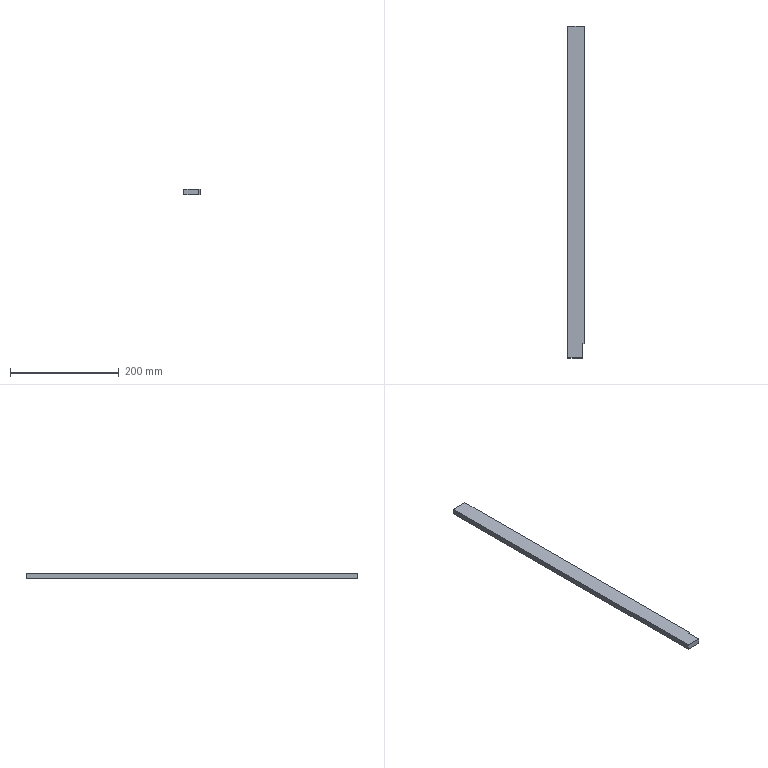Part | SolidWorks | features Extrusion 1, ICE 1 | 1 solid | 8 faces | box 30 x 610 x 10 mm | volume 182220 mm3 | plane 8
STEP:
#1=CARTESIAN_POINT('',(0.,0.,0.));
#2=VERTEX_POINT('',#1);
#3=CARTESIAN_POINT('',(0.,-610.,0.));
#4=VERTEX_POINT('',#3);
#5=CARTESIAN_POINT('',(0.,0.,0.));
#6=DIRECTION('',(0.,-1.,0.));
#7=VECTOR('',#6,1000.);
#8=LINE('',#5,#7);
#9=EDGE_CURVE('',#2,#4,#8,.T.);
#10=ORIENTED_EDGE('',*,*,#9,.T.);
#11=CARTESIAN_POINT('',(0.,-610.,10.));
#12=VERTEX_POINT('',#11);
#13=CARTESIAN_POINT('',(0.,-610.,10.));
#14=DIRECTION('',(0.,0.,-1.));
#15=VECTOR('',#14,1000.);
#16=LINE('',#13,#15);
#17=EDGE_CURVE('',#12,#4,#16,.T.);
#18=ORIENTED_EDGE('',*,*,#17,.F.);
#19=CARTESIAN_POINT('',(0.,0.,10.));
#20=VERTEX_POINT('',#19);
#21=CARTESIAN_POINT('',(0.,0.,10.));
#22=DIRECTION('',(0.,-1.,0.));
#23=VECTOR('',#22,1000.);
#24=LINE('',#21,#23);
#25=EDGE_CURVE('',#20,#12,#24,.T.);
#26=ORIENTED_EDGE('',*,*,#25,.F.);
#27=CARTESIAN_POINT('',(0.,0.,10.));
#28=DIRECTION('',(0.,0.,-1.));
#29=VECTOR('',#28,1000.);
#30=LINE('',#27,#29);
#31=EDGE_CURVE('',#20,#2,#30,.T.);
#32=ORIENTED_EDGE('',*,*,#31,.T.);
#33=EDGE_LOOP('',(#10,#18,#26,#32));
#34=FACE_OUTER_BOUND('',#33,.T.);
#35=CARTESIAN_POINT('',(0.,0.,10.));
#36=DIRECTION('',(1.,0.,0.));
#37=DIRECTION('',(0.,0.,-1.));
#38=AXIS2_PLACEMENT_3D('',#35,#36,#37);
#39=PLANE('',#38);
#40=ADVANCED_FACE('',(#34),#39,.F.);
#41=CARTESIAN_POINT('',(27.,-610.,0.));
#42=VERTEX_POINT('',#41);
#43=CARTESIAN_POINT('',(0.,-610.,0.));
#44=DIRECTION('',(1.,0.,0.));
#45=VECTOR('',#44,1000.);
#46=LINE('',#43,#45);
#47=EDGE_CURVE('',#4,#42,#46,.T.);
#48=ORIENTED_EDGE('',*,*,#47,.T.);
#49=CARTESIAN_POINT('',(27.,-610.,10.));
#50=VERTEX_POINT('',#49);
#51=CARTESIAN_POINT('',(27.,-610.,0.));
#52=DIRECTION('',(0.,0.,1.));
#53=VECTOR('',#52,1000.);
#54=LINE('',#51,#53);
#55=EDGE_CURVE('',#42,#50,#54,.T.);
#56=ORIENTED_EDGE('',*,*,#55,.T.);
#57=CARTESIAN_POINT('',(0.,-610.,10.));
#58=DIRECTION('',(1.,0.,0.));
#59=VECTOR('',#58,1000.);
#60=LINE('',#57,#59);
#61=EDGE_CURVE('',#12,#50,#60,.T.);
#62=ORIENTED_EDGE('',*,*,#61,.F.);
#63=ORIENTED_EDGE('',*,*,#17,.T.);
#64=EDGE_LOOP('',(#48,#56,#62,#63));
#65=FACE_OUTER_BOUND('',#64,.T.);
#66=CARTESIAN_POINT('',(0.,-610.,10.));
#67=DIRECTION('',(0.,1.,0.));
#68=DIRECTION('',(0.,0.,1.));
#69=AXIS2_PLACEMENT_3D('',#66,#67,#68);
#70=PLANE('',#69);
#71=ADVANCED_FACE('',(#65),#70,.F.);
#72=CARTESIAN_POINT('',(30.,-584.,10.));
#73=VERTEX_POINT('',#72);
#74=CARTESIAN_POINT('',(30.,0.,10.));
#75=VERTEX_POINT('',#74);
#76=CARTESIAN_POINT('',(30.,0.,10.));
#77=DIRECTION('',(0.,1.,0.));
#78=VECTOR('',#77,1000.);
#79=LINE('',#76,#78);
#80=EDGE_CURVE('',#73,#75,#79,.T.);
#81=ORIENTED_EDGE('',*,*,#80,.F.);
#82=CARTESIAN_POINT('',(30.,-584.,0.));
#83=VERTEX_POINT('',#82);
#84=CARTESIAN_POINT('',(30.,-584.,0.));
#85=DIRECTION('',(0.,0.,1.));
#86=VECTOR('',#85,1000.);
#87=LINE('',#84,#86);
#88=EDGE_CURVE('',#83,#73,#87,.T.);
#89=ORIENTED_EDGE('',*,*,#88,.F.);
#90=CARTESIAN_POINT('',(30.,0.,0.));
#91=VERTEX_POINT('',#90);
#92=CARTESIAN_POINT('',(30.,0.,0.));
#93=DIRECTION('',(0.,1.,0.));
#94=VECTOR('',#93,1000.);
#95=LINE('',#92,#94);
#96=EDGE_CURVE('',#83,#91,#95,.T.);
#97=ORIENTED_EDGE('',*,*,#96,.T.);
#98=CARTESIAN_POINT('',(30.,0.,10.));
#99=DIRECTION('',(0.,0.,-1.));
#100=VECTOR('',#99,1000.);
#101=LINE('',#98,#100);
#102=EDGE_CURVE('',#75,#91,#101,.T.);
#103=ORIENTED_EDGE('',*,*,#102,.F.);
#104=EDGE_LOOP('',(#81,#89,#97,#103));
#105=FACE_OUTER_BOUND('',#104,.T.);
#106=CARTESIAN_POINT('',(30.,0.,10.));
#107=DIRECTION('',(-1.,0.,0.));
#108=DIRECTION('',(0.,-1.,0.));
#109=AXIS2_PLACEMENT_3D('',#106,#107,#108);
#110=PLANE('',#109);
#111=ADVANCED_FACE('',(#105),#110,.F.);
#112=CARTESIAN_POINT('',(0.,0.,0.));
#113=DIRECTION('',(-1.,0.,0.));
#114=VECTOR('',#113,1000.);
#115=LINE('',#112,#114);
#116=EDGE_CURVE('',#91,#2,#115,.T.);
#117=ORIENTED_EDGE('',*,*,#116,.T.);
#118=ORIENTED_EDGE('',*,*,#31,.F.);
#119=CARTESIAN_POINT('',(0.,0.,10.));
#120=DIRECTION('',(-1.,0.,0.));
#121=VECTOR('',#120,1000.);
#122=LINE('',#119,#121);
#123=EDGE_CURVE('',#75,#20,#122,.T.);
#124=ORIENTED_EDGE('',*,*,#123,.F.);
#125=ORIENTED_EDGE('',*,*,#102,.T.);
#126=EDGE_LOOP('',(#117,#118,#124,#125));
#127=FACE_OUTER_BOUND('',#126,.T.);
#128=CARTESIAN_POINT('',(0.,0.,10.));
#129=DIRECTION('',(0.,-1.,0.));
#130=DIRECTION('',(0.,0.,-1.));
#131=AXIS2_PLACEMENT_3D('',#128,#129,#130);
#132=PLANE('',#131);
#133=ADVANCED_FACE('',(#127),#132,.F.);
#134=CARTESIAN_POINT('',(27.,-584.,10.));
#135=VERTEX_POINT('',#134);
#136=CARTESIAN_POINT('',(27.,-610.,10.));
#137=DIRECTION('',(0.,-1.,0.));
#138=VECTOR('',#137,1000.);
#139=LINE('',#136,#138);
#140=EDGE_CURVE('',#135,#50,#139,.T.);
#141=ORIENTED_EDGE('',*,*,#140,.F.);
#142=CARTESIAN_POINT('',(30.,-584.,10.));
#143=DIRECTION('',(-1.,0.,0.));
#144=VECTOR('',#143,1000.);
#145=LINE('',#142,#144);
#146=EDGE_CURVE('',#73,#135,#145,.T.);
#147=ORIENTED_EDGE('',*,*,#146,.F.);
#148=ORIENTED_EDGE('',*,*,#80,.T.);
#149=ORIENTED_EDGE('',*,*,#123,.T.);
#150=ORIENTED_EDGE('',*,*,#25,.T.);
#151=ORIENTED_EDGE('',*,*,#61,.T.);
#152=EDGE_LOOP('',(#141,#147,#148,#149,#150,#151));
#153=FACE_OUTER_BOUND('',#152,.T.);
#154=CARTESIAN_POINT('',(0.,0.,10.));
#155=DIRECTION('',(0.,0.,1.));
#156=DIRECTION('',(1.,0.,0.));
#157=AXIS2_PLACEMENT_3D('',#154,#155,#156);
#158=PLANE('',#157);
#159=ADVANCED_FACE('',(#153),#158,.T.);
#160=CARTESIAN_POINT('',(27.,-584.,0.));
#161=VERTEX_POINT('',#160);
#162=CARTESIAN_POINT('',(30.,-584.,0.));
#163=DIRECTION('',(-1.,0.,0.));
#164=VECTOR('',#163,1000.);
#165=LINE('',#162,#164);
#166=EDGE_CURVE('',#83,#161,#165,.T.);
#167=ORIENTED_EDGE('',*,*,#166,.T.);
#168=CARTESIAN_POINT('',(27.,-610.,0.));
#169=DIRECTION('',(0.,-1.,0.));
#170=VECTOR('',#169,1000.);
#171=LINE('',#168,#170);
#172=EDGE_CURVE('',#161,#42,#171,.T.);
#173=ORIENTED_EDGE('',*,*,#172,.T.);
#174=ORIENTED_EDGE('',*,*,#47,.F.);
#175=ORIENTED_EDGE('',*,*,#9,.F.);
#176=ORIENTED_EDGE('',*,*,#116,.F.);
#177=ORIENTED_EDGE('',*,*,#96,.F.);
#178=EDGE_LOOP('',(#167,#173,#174,#175,#176,#177));
#179=FACE_OUTER_BOUND('',#178,.T.);
#180=CARTESIAN_POINT('',(0.,0.,0.));
#181=DIRECTION('',(0.,0.,1.));
#182=DIRECTION('',(1.,0.,0.));
#183=AXIS2_PLACEMENT_3D('',#180,#181,#182);
#184=PLANE('',#183);
#185=ADVANCED_FACE('',(#179),#184,.F.);
#186=ORIENTED_EDGE('',*,*,#140,.T.);
#187=ORIENTED_EDGE('',*,*,#55,.F.);
#188=ORIENTED_EDGE('',*,*,#172,.F.);
#189=CARTESIAN_POINT('',(27.,-584.,0.));
#190=DIRECTION('',(0.,0.,1.));
#191=VECTOR('',#190,1000.);
#192=LINE('',#189,#191);
#193=EDGE_CURVE('',#161,#135,#192,.T.);
#194=ORIENTED_EDGE('',*,*,#193,.T.);
#195=EDGE_LOOP('',(#186,#187,#188,#194));
#196=FACE_OUTER_BOUND('',#195,.T.);
#197=CARTESIAN_POINT('',(27.,-610.,0.));
#198=DIRECTION('',(-1.,0.,0.));
#199=DIRECTION('',(0.,0.,1.));
#200=AXIS2_PLACEMENT_3D('',#197,#198,#199);
#201=PLANE('',#200);
#202=ADVANCED_FACE('',(#196),#201,.F.);
#203=ORIENTED_EDGE('',*,*,#146,.T.);
#204=ORIENTED_EDGE('',*,*,#193,.F.);
#205=ORIENTED_EDGE('',*,*,#166,.F.);
#206=ORIENTED_EDGE('',*,*,#88,.T.);
#207=EDGE_LOOP('',(#203,#204,#205,#206));
#208=FACE_OUTER_BOUND('',#207,.T.);
#209=CARTESIAN_POINT('',(30.,-584.,0.));
#210=DIRECTION('',(0.,1.,0.));
#211=DIRECTION('',(0.,0.,1.));
#212=AXIS2_PLACEMENT_3D('',#209,#210,#211);
#213=PLANE('',#212);
#214=ADVANCED_FACE('',(#208),#213,.F.);
#215=CLOSED_SHELL('',(#40,#71,#111,#133,#159,#185,#202,#214));
#216=MANIFOLD_SOLID_BREP('',#215);
#217=CARTESIAN_POINT('',(0.,0.,0.));
#218=DIRECTION('',(0.,0.,1.));
#219=DIRECTION('',(1.,0.,0.));
#220=AXIS2_PLACEMENT_3D('',#217,#218,#219);
#221=(LENGTH_UNIT()NAMED_UNIT(*)SI_UNIT(.MILLI.,.METRE.));
#222=UNCERTAINTY_MEASURE_WITH_UNIT(LENGTH_MEASURE(0.00001),#221,'','');
#223=(NAMED_UNIT(*)PLANE_ANGLE_UNIT()SI_UNIT($,.RADIAN.));
#224=(NAMED_UNIT(*)SI_UNIT($,.STERADIAN.)SOLID_ANGLE_UNIT());
#225=(GEOMETRIC_REPRESENTATION_CONTEXT(3)GLOBAL_UNCERTAINTY_ASSIGNED_CONTEXT((#222))GLOBAL_UNIT_ASSIGNED_CONTEXT((#221,#223,#224))REPRESENTATION_CONTEXT('',''));
#226=ADVANCED_BREP_SHAPE_REPRESENTATION('',(#216,#220),#225);